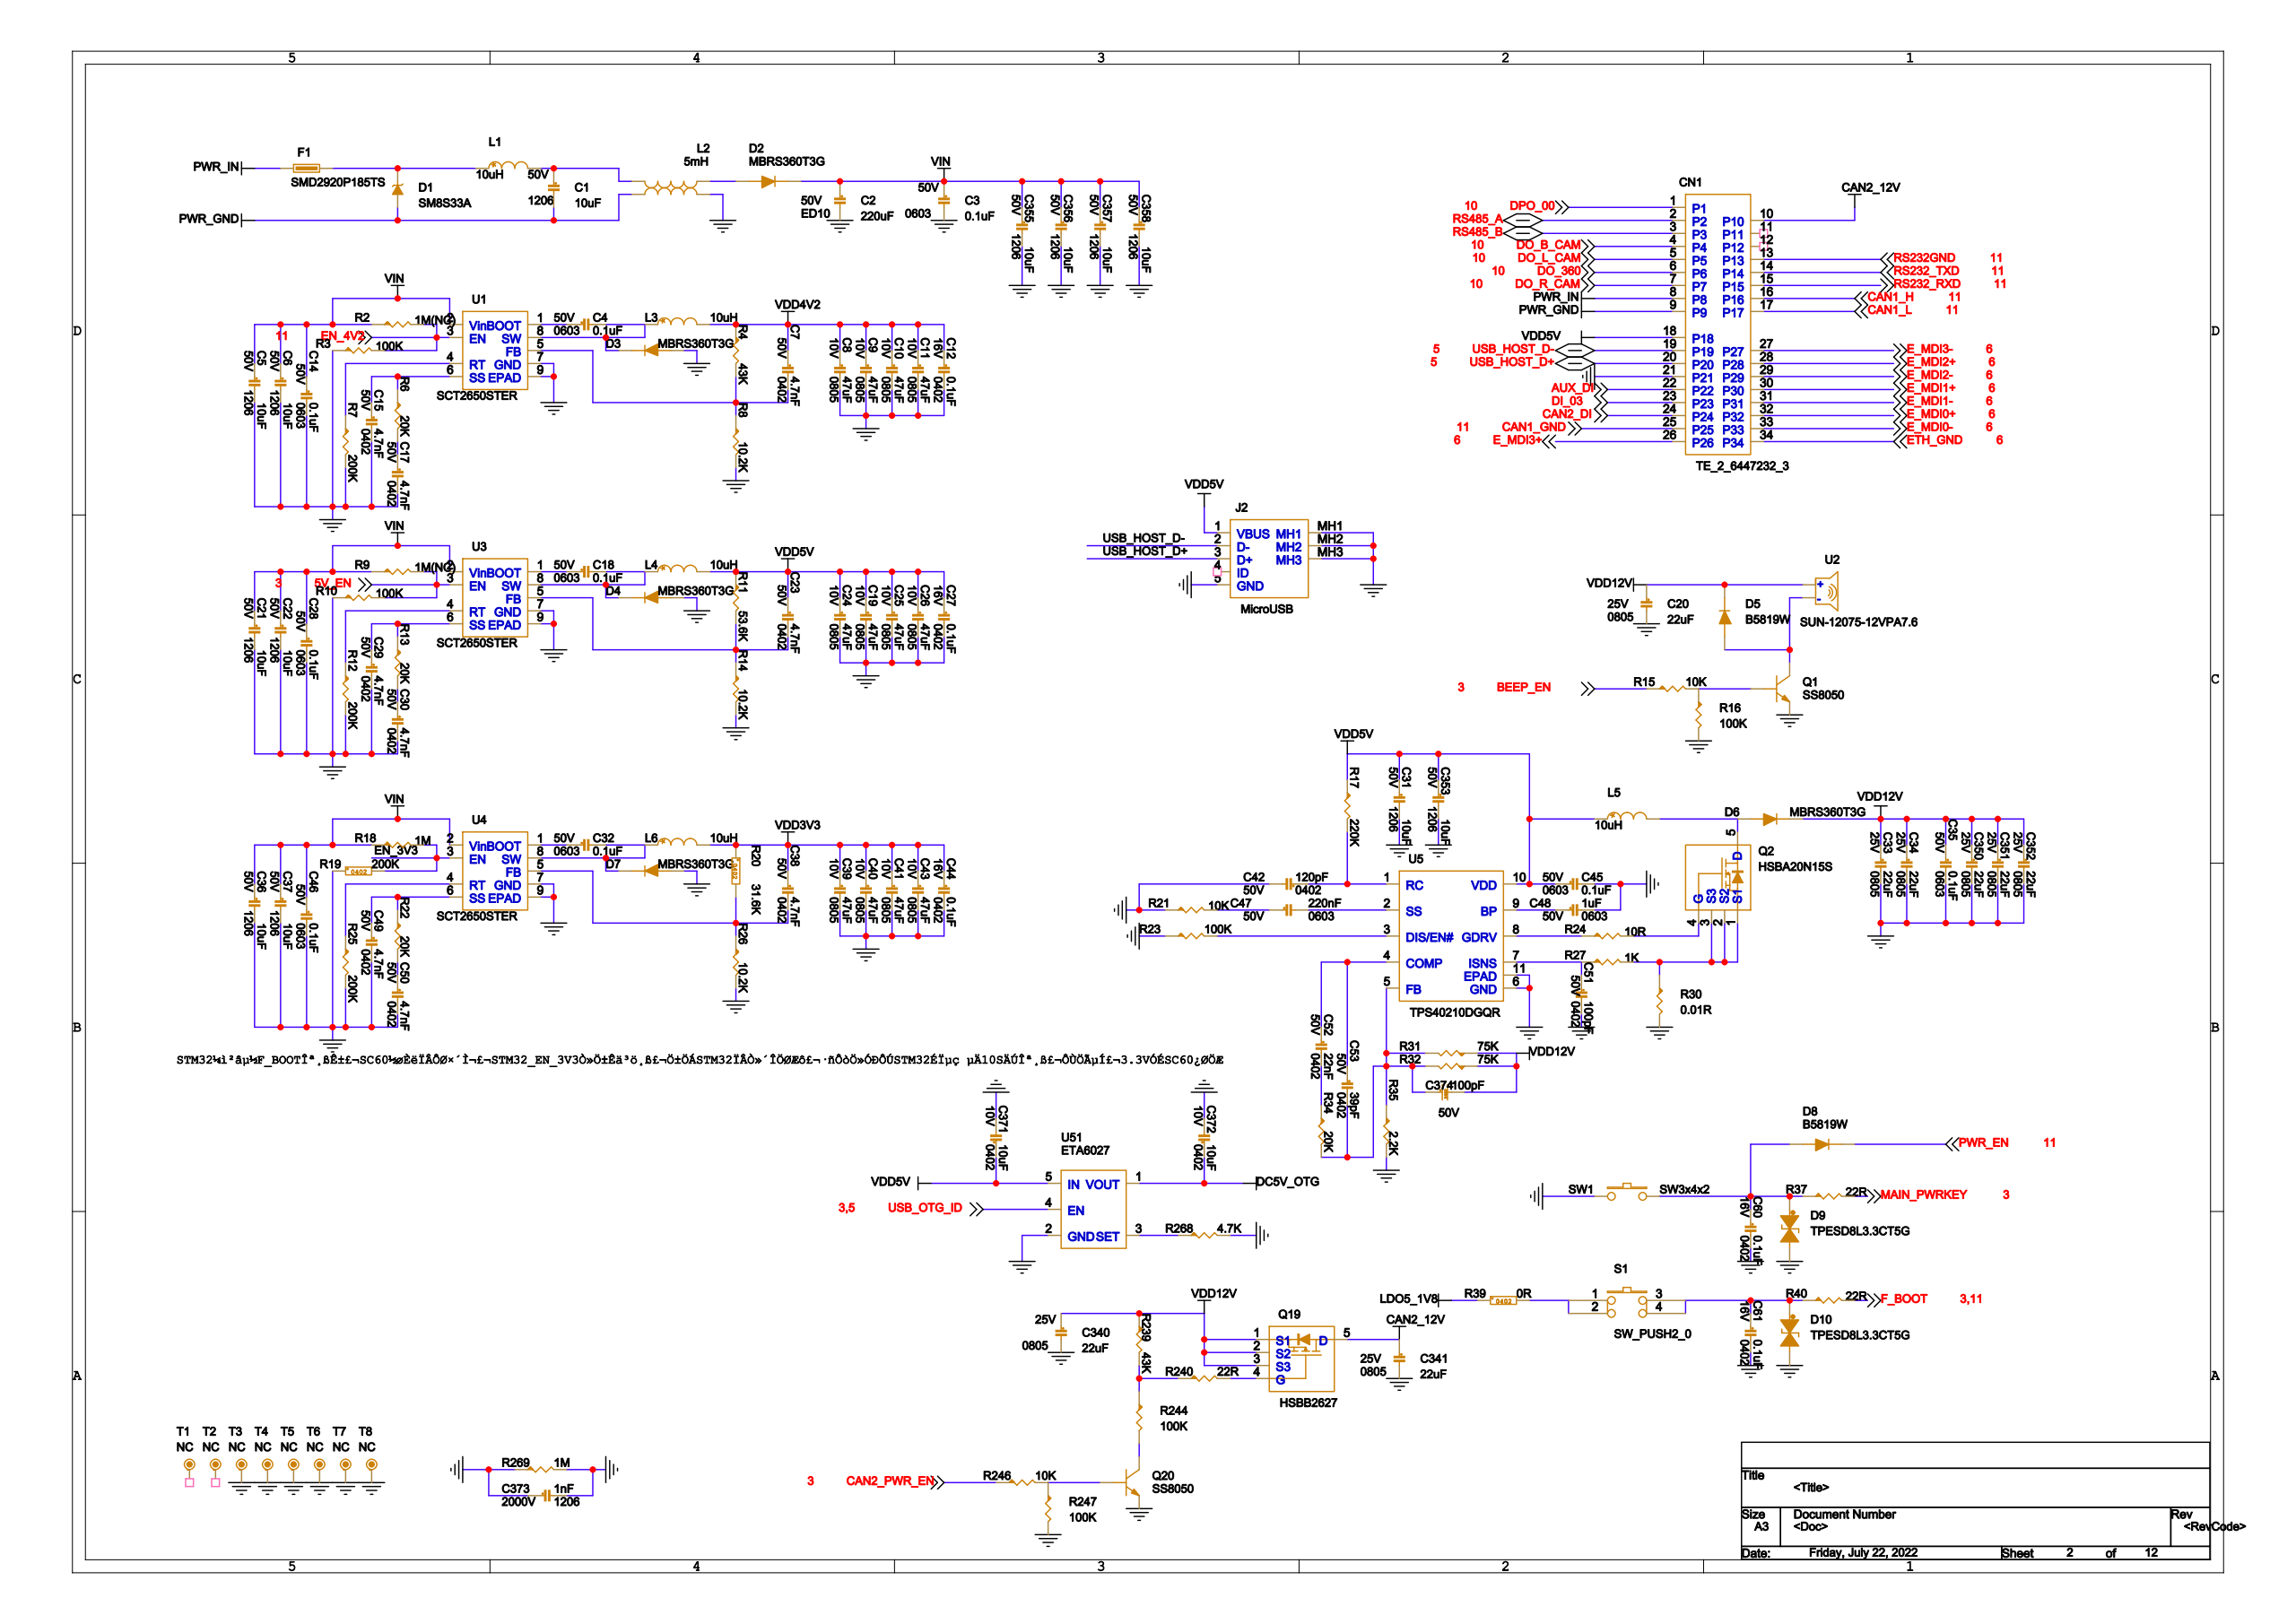Circuit board | Cadence Allegro | 970 parts | 627 nets | one sheet of the schematic
Parts on this sheet (reference | value | footprint):
C1 | 10uF | C1206
C2 | 220uF | ED10
C5 | 10uF | C1206
C6 | 10uF | C1206
C7 | 4.7nF | C0402
C8 | 47uF | C0805
C9 | 47uF | C0805
C10 | 47uF | C0805
C11 | 47uF | C0805
C12 | 0.1uF | C0402
C14 | 0.1uF | C0603
C15 | 4.7nF | C0402
C17 | 4.7nF | C0402
C18 | 0.1uF | C0603
C19 | 47uF | C0805
C20 | 22uF | C0805
C21 | 10uF | C1206
C22 | 10uF | C1206
C23 | 4.7nF | C0402
C24 | 47uF | C0805
C25 | 47uF | C0805
C26 | 47uF | C0805
C27 | 0.1uF | C0402
C28 | 0.1uF | C0603
C29 | 4.7nF | C0402
C30 | 4.7nF | C0402
C31 | 10uF | C1206
C32 | 0.1uF | C0603
C33 | 22uF | C0805
C34 | 22uF | C0805
C35 | 0.1uF | C0603
C36 | 10uF | C1206
C37 | 10uF | C1206
C38 | 4.7nF | C0402
C39 | 47uF | C0805
C40 | 47uF | C0805
C41 | 47uF | C0805
C42 | 120pF | C0402
C43 | 47uF | C0805
C44 | 0.1uF | C0402
C45 | 0.1uF | C0603
C46 | 0.1uF | C0603
C47 | 220nF | C0603
C48 | 1uF | C0603
C49 | 4.7nF | C0402
C50 | 4.7nF | C0402
C51 | 100pF | C0402
C52 | 22nF | C0402
C53 | 39pF | C0402
C60 | 0.1uF | C0402
C61 | 0.1uF | C0402
C340 | 22uF | C0805
C341 | 22uF | C0805
C350 | 22uF | C0805
C351 | 22uF | C0805
C352 | 22uF | C0805
C353 | 10uF | C1206
C355 | 10uF | C1206
C356 | 10uF | C1206
C357 | 10uF | C1206
C358 | 10uF | C1206
C371 | 10uF | C0402
C372 | 10uF | C0402
C373 | 1nF | C1206
CN1 | TE_2_6447232_3 | TE_2-6447232-3
D1 | SM8S33A | DO_218AB
D2 | MBRS360T3G | SMC
D3 | MBRS360T3G | SMC
D4 | MBRS360T3G | SMC
D5 | B5819W | SOD-123
D6 | MBRS360T3G | SMC
D7 | MBRS360T3G | SMC
D8 | B5819W | SOD-123
D9 | TPESD8L3.3CT5G | DFN1006_2L
D10 | TPESD8L3.3CT5G | DFN1006_2L
F1 | SMD2920P185TS | R2920
J2 | MicroUSB | MICROUSB_180_SMD
L1 | 10uH | IND0630
L2 | 5mH | SQ1212WS
L3 | 10uH | L10X10
L4 | 10uH | L10X10
L5 | 10uH | IND0630
L6 | 10uH | L10X10
Q1 | SS8050 | SOT-23
Q2 | HSBA20N15S | DFN5X6
Q19 | HSBB2627 | DFN3X3
Q20 | SS8050 | SOT-23
R2 | 1M(NC) | R0402
R3 | 100K | R0402
R4 | 43K | R0402
R6 | 20K | R0402
R7 | 200K | R0402
R8 | 10.2K | R0402
R9 | 1M(NC) | R0402
R10 | 100K | R0402
R11 | 53.6K | R0402
R12 | 200K | R0402
R13 | 20K | R0402
R14 | 10.2K | R0402
R15 | 10K | R0402
R16 | 100K | R0402
R17 | 220K | R0402
R18 | 1M | R0402
R19 | 200K | R0402
R20 | 31.6K | R0402
R21 | 10K | R0402
R22 | 20K | R0402
R23 | 100K | R0402
R24 | 10R | R0402
R25 | 200K | R0402
R26 | 10.2K | R0402
R27 | 1K | R0402
R30 | 0.01R | R2512
R31 | 75K | R0402
R32 | 75K | R0402
R34 | 20K | R0402
R35 | 2.2K | R0402
R37 | 22R | R0402
R39 | 0R | R0402
R40 | 22R | R0402
R239 | 43K | R0402
R240 | 22R | R0402
R244 | 100K | R0402
R246 | 10K | R0402
R247 | 100K | R0402
R268 | 4.7K | R0402
R269 | 1M | R1206
S1 | SW_PUSH2_0 | SW_6X6
SW1 | SW3x4x2 | SW3X4X2
T3 | NC | M3
T4 | NC | M3
T5 | NC | M3
T6 | NC | M3
T7 | NC | M3
T8 | NC | M3
U1 | SCT2650STER | SO8_EPAD
U2 | SUN-12075-12VPA7.6 | BEEP_7P6_12
U3 | SCT2650STER | SO8_EPAD
U4 | SCT2650STER | SO8_EPAD
U5 | TPS40210DGQR | HVSSOP10
U51 | ETA6027 | SOT23-5
Nets of these parts (net: part-pin ...):
VDD5V: C19-1 C23-1 C24-1 C25-1 C26-1 C27-1 C31-1 C45-1 C353-1 C371-1 J2-1 L4-2 L5-1 R11-1 R17-1 U5-10 U51-5 CN1-18
VDD3V3: C38-1 C39-1 C40-1 C41-1 C43-1 C44-1 L6-2 R20-1
GND: C2-2 C5-2 C6-2 C8-2 C9-2 C10-2 C11-2 C12-2 C14-2 C15-2 C17-2 C19-2 C20-2 C21-2 C22-2 C24-2 C25-2 C26-2 C27-2 C28-2 C29-2 C30-2 C31-2 C33-2 C34-2 C35-2 C36-2 C37-2 C39-2 C40-2 C41-2 C42-2 C43-2 C44-2 C45-2 C46-2 C48-2 C49-2 C50-2 C51-2 C60-2 C61-2 C340-2 C341-2 C350-2 C351-2 C352-2 C353-2 C355-2 C356-2 C357-2 C358-2 C371-2 C372-2 C373-1 D3-1 D4-1 D7-1 D9-1 D10-1 J2-5 J2-MH1 J2-MH2 J2-MH3 L2-3 Q1-2 Q20-2 R3-1 R7-2 R8-2 R10-1 R12-2 R14-2 R16-2 R19-1 R21-1 R23-1 R25-2 R26-2 R30-2 R35-2 R247-2 R268-2 R269-1 SW1-1 U1-7 U1-9 U3-7 U3-9 U4-7 U4-9 U5-6 U5-11 U51-2 CN1-21
N19188620: D3-2 L3-1 U1-8
VDD4V2: C7-1 C8-1 C9-1 C10-1 C11-1 C12-1 L3-2 R4-1
N19192194: C18-2 D4-2 L4-1 U3-8
N19419768: C32-2 D7-2 L6-1 U4-8
PWR_IN: F1-1 CN1-8
CAN2_DI: CN1-24
E_MDI1+: CN1-30
E_MDI1-: CN1-31
E_MDI0+: CN1-32
E_MDI0-: CN1-33
AUX_DI: CN1-22
N19214172: C53-2 R31-2 R32-2 R34-2 R35-1 U5-5
VDD12V: C20-1 C33-1 C34-1 C35-1 C340-1 C350-1 C351-1 C352-1 D5-2 D6-2 Q19-1 Q19-2 Q19-3 R31-1 R32-1 R239-1 U2-1
DI_03: CN1-23
USB_HOST_D+: J2-3 CN1-20
USB_HOST_D-: J2-2 CN1-19
EN_3V3: R18-2 R19-2 U4-3
N19419806: C38-2 R20-2 R26-1 U4-5
LDO5_1V8: R39-1
N19210085: R39-2 S1-1 S1-2
USB_OTG_ID: U51-4
N19192240: C23-2 R11-2 R14-1 U3-5
EGND: C373-2 R269-2 T3-1 T4-1 T5-1 T6-1 T7-1 T8-1
DPO_00: CN1-1
CAN2_12V: C341-1 Q19-5 CN1-10
RS232GND: CN1-13
RS232_TXD: CN1-14
RS232_RXD: CN1-15
CAN1_H: CN1-16
CAN1_L: CN1-17
RS485_A: CN1-2
CAN1_GND: CN1-25
E_MDI3+: CN1-26
E_MDI3-: CN1-27
E_MDI2+: CN1-28
E_MDI2-: CN1-29
RS485_B: CN1-3
ETH_GND: CN1-34
DO_B_CAM: CN1-4
DO_L_CAM: CN1-5
DO_360: CN1-6
DO_R_CAM: CN1-7
PWR_GND: C1-2 D1-1 L2-4 CN1-9
VIN: C2-1 C5-1 C6-1 C14-1 C21-1 C22-1 C28-1 C36-1 C37-1 C46-1 C355-1 C356-1 C357-1 C358-1 D2-2 R2-1 R9-1 R18-1 U1-2 U3-2 U4-2
N19188183: C1-1 L1-2 L2-2
N19212613: C47-1 R21-2
N19212576: C47-2 U5-2
N19215705: C48-1 U5-9
N19419766: C32-1 U4-1
N19192192: C18-1 U3-1
N19188617: U1-1
N19419904: C50-1 R22-2
N19419708: C49-1 R22-1 U4-6
N19188418: C15-1 R6-1 U1-6
N19190211: C17-1 R6-2
N19192142: C29-1 R13-1 U3-6
N19192350: C30-1 R13-2
N19188753: C7-2 R4-2 R8-1 U1-5
N19216205: C51-1 R27-1 U5-7
N19212556: C42-1 R17-2 U5-1
N19214126: C52-1 C53-1 U5-4
N19214169: C52-2 R34-1
N19188121: D1-2 F1-2 L1-1
N19208937: C61-1 D10-2 R40-1 S1-3 S1-4
N19209763: C60-1 D8-1 D9-2 R37-1 SW1-2
F_BOOT: R40-2
PWR_EN: D8-2
DC5V_OTG: C372-1 U51-1
N19307961: D5-1 Q1-3 U2-2
N19188266: D2-1 L2-1
N19216580: D6-1 L5-2 Q2-5
N19307951: Q1-1 R15-2 R16-1
N19743207: Q20-1 R246-2 R247-1
N19743230: Q20-3 R244-2
N19743240: Q19-4 R240-2
N19216533: Q2-4 R24-2
N19216509: Q2-1 Q2-2 Q2-3 R27-2 R30-1
5V_EN: R9-2 R10-2 U3-3
N19212610: R23-2 U5-3
N19743184: R239-2 R240-1 R244-1
EN_4V2: R2-2 R3-2 U1-3
N19591108: R268-1 U51-3
MAIN_PWRKEY: R37-2
BEEP_EN: R15-1
CAN2_PWR_EN: R246-1
N19419704: R25-1 U4-4
N19192130: R12-1 U3-4
N19188400: R7-1 U1-4
N19216208: R24-1 U5-8